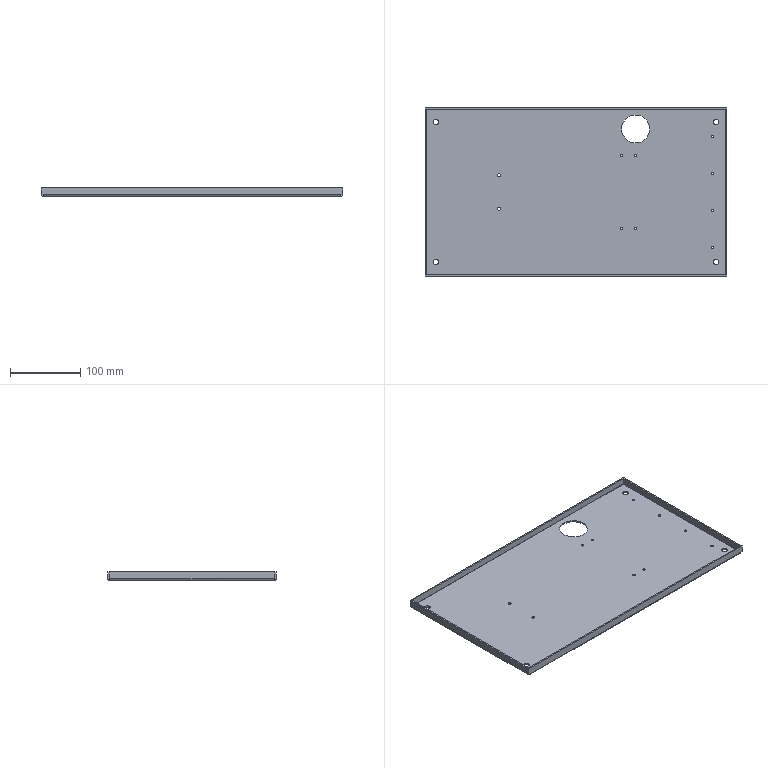Part | STEP file | CS-DS-003 | 1 solid | 76 faces | box 430 x 240 x 12 mm | volume 228512 mm3 | cylinder 38 | plane 30 | spline 8 | commonest cylinder face diameters 3.3 x16 8 x8 0.4 x4 4.2 x4 4.4 x4 40 x2